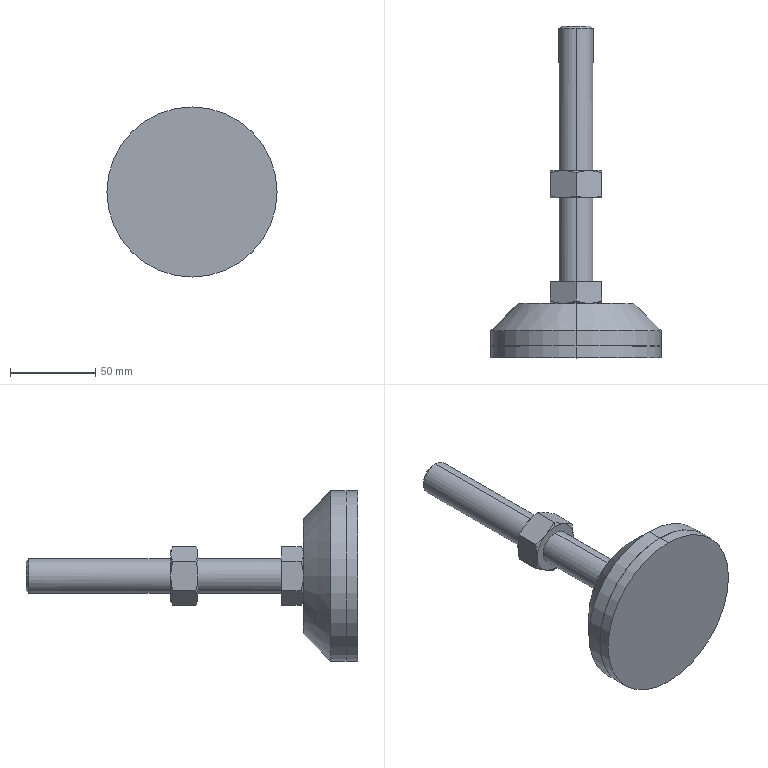Part | SolidWorks | features BaseBody 2, LPattern 1 | 2 solids | 59 faces | box 100 x 195 x 100 mm | volume 281117 mm3 | cone 29 | plane 20 | cylinder 10 | commonest cylinder face diameters 100 x4 17.294 x2 20 x2 99.9 x2